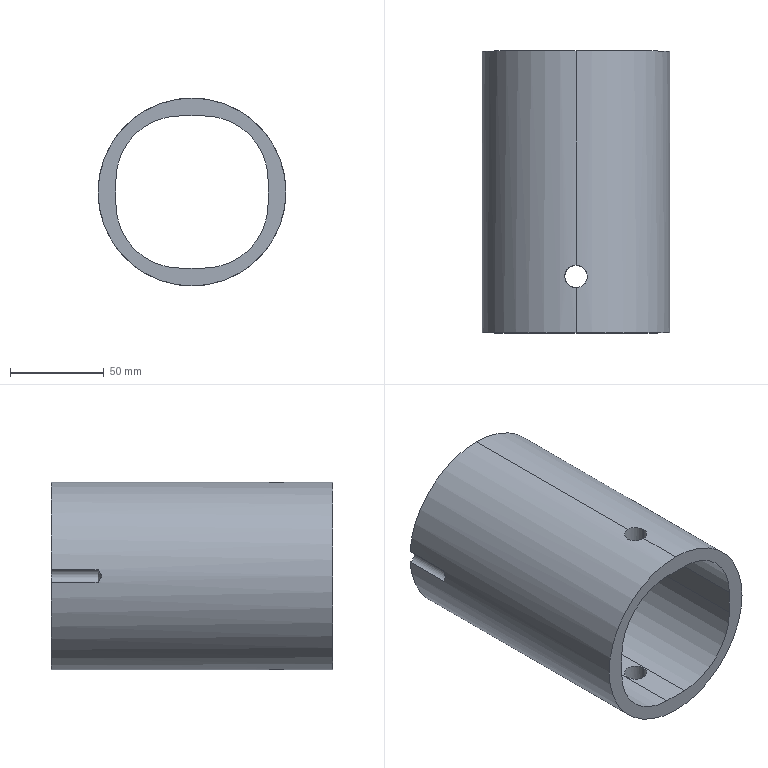Part | SolidWorks | features MirrorStock 1 | 1 solid | 20 faces | box 100 x 150 x 100 mm | volume 339747 mm3 | cylinder 12 | plane 6 | cone 2 | commonest cylinder face diameters 12 x4 68 x4 6.8 x2 100 x2
STEP:
#1=CARTESIAN_POINT('',(-6.,-45.,-40.5));
#2=VERTEX_POINT('',#1);
#3=CARTESIAN_POINT('',(6.,-45.,-40.5));
#4=VERTEX_POINT('',#3);
#5=CARTESIAN_POINT('',(0.,-45.,-40.5));
#6=DIRECTION('',(0.,0.,-1.));
#7=DIRECTION('',(-1.,0.,0.));
#8=AXIS2_PLACEMENT_3D('',#5,#6,#7);
#9=CIRCLE('',#8,6.);
#10=EDGE_CURVE('',#2,#4,#9,.T.);
#11=ORIENTED_EDGE('',*,*,#10,.F.);
#12=CARTESIAN_POINT('',(-6.,-45.,-49.639));
#13=VERTEX_POINT('',#12);
#14=CARTESIAN_POINT('',(-6.,-45.,75.));
#15=DIRECTION('',(0.,0.,-1.));
#16=VECTOR('',#15,1000.);
#17=LINE('',#14,#16);
#18=EDGE_CURVE('',#2,#13,#17,.T.);
#19=ORIENTED_EDGE('',*,*,#18,.T.);
#20=CARTESIAN_POINT('',(0.,-39.,-50.));
#21=VERTEX_POINT('',#20);
#22=CARTESIAN_POINT('',(-6.,-45.,-49.639));
#23=CARTESIAN_POINT('',(-6.,-44.608,-49.639));
#24=CARTESIAN_POINT('',(-5.962,-44.218,-49.643));
#25=CARTESIAN_POINT('',(-5.847,-43.637,-49.657));
#26=CARTESIAN_POINT('',(-5.798,-43.444,-49.663));
#27=CARTESIAN_POINT('',(-5.684,-43.068,-49.676));
#28=CARTESIAN_POINT('',(-5.552,-42.7,-49.691));
#29=CARTESIAN_POINT('',(-5.385,-42.346,-49.709));
#30=CARTESIAN_POINT('',(-5.2,-42.,-49.729));
#31=CARTESIAN_POINT('',(-5.098,-41.829,-49.74));
#32=CARTESIAN_POINT('',(-4.769,-41.337,-49.773));
#33=CARTESIAN_POINT('',(-4.521,-41.035,-49.796));
#34=CARTESIAN_POINT('',(-3.967,-40.482,-49.843));
#35=CARTESIAN_POINT('',(-3.659,-40.229,-49.867));
#36=CARTESIAN_POINT('',(-3.007,-39.793,-49.911));
#37=CARTESIAN_POINT('',(-2.663,-39.609,-49.93));
#38=CARTESIAN_POINT('',(-2.117,-39.383,-49.955));
#39=CARTESIAN_POINT('',(-1.93,-39.315,-49.963));
#40=CARTESIAN_POINT('',(-1.553,-39.201,-49.976));
#41=CARTESIAN_POINT('',(-1.363,-39.154,-49.982));
#42=CARTESIAN_POINT('',(-0.7871,-39.039,-49.995));
#43=CARTESIAN_POINT('',(-0.3969,-39.,-50.));
#44=CARTESIAN_POINT('',(0.,-39.,-50.));
#45=B_SPLINE_CURVE_WITH_KNOTS('',3,(#22,#23,#24,#25,#26,#27,#28,#29,#30,#31,#32,#33,#34,#35,#36,#37,#38,#39,#40,#41,#42,#43,#44),.UNSPECIFIED.,.F.,.F.,(4,2,2,1,2,2,2,2,2,2,2,4),(0.01878,0.01995,0.02054,0.02112,0.02171,0.0223,0.02347,0.02464,0.02582,0.0264,0.02699,0.02817),.UNSPECIFIED.);
#46=EDGE_CURVE('',#13,#21,#45,.T.);
#47=ORIENTED_EDGE('',*,*,#46,.T.);
#48=CARTESIAN_POINT('',(6.,-45.,-49.639));
#49=VERTEX_POINT('',#48);
#50=CARTESIAN_POINT('',(0.,-39.,-50.));
#51=CARTESIAN_POINT('',(0.3965,-39.,-50.));
#52=CARTESIAN_POINT('',(0.7864,-39.039,-49.995));
#53=CARTESIAN_POINT('',(1.362,-39.153,-49.982));
#54=CARTESIAN_POINT('',(1.552,-39.201,-49.976));
#55=CARTESIAN_POINT('',(1.929,-39.315,-49.963));
#56=CARTESIAN_POINT('',(2.116,-39.382,-49.956));
#57=CARTESIAN_POINT('',(2.66,-39.608,-49.93));
#58=CARTESIAN_POINT('',(3.005,-39.792,-49.911));
#59=CARTESIAN_POINT('',(3.657,-40.227,-49.867));
#60=CARTESIAN_POINT('',(3.965,-40.48,-49.843));
#61=CARTESIAN_POINT('',(4.518,-41.032,-49.796));
#62=CARTESIAN_POINT('',(4.766,-41.334,-49.773));
#63=CARTESIAN_POINT('',(5.095,-41.825,-49.74));
#64=CARTESIAN_POINT('',(5.197,-41.995,-49.729));
#65=CARTESIAN_POINT('',(5.382,-42.341,-49.71));
#66=CARTESIAN_POINT('',(5.466,-42.517,-49.7));
#67=CARTESIAN_POINT('',(5.691,-43.058,-49.675));
#68=CARTESIAN_POINT('',(5.806,-43.436,-49.662));
#69=CARTESIAN_POINT('',(5.961,-44.211,-49.643));
#70=CARTESIAN_POINT('',(6.,-44.603,-49.639));
#71=CARTESIAN_POINT('',(6.,-45.,-49.639));
#72=B_SPLINE_CURVE_WITH_KNOTS('',3,(#50,#51,#52,#53,#54,#55,#56,#57,#58,#59,#60,#61,#62,#63,#64,#65,#66,#67,#68,#69,#70,#71),.UNSPECIFIED.,.F.,.F.,(4,2,2,2,2,2,2,2,2,2,4),(0.02817,0.02934,0.02992,0.03051,0.03168,0.03286,0.03403,0.03462,0.0352,0.03637,0.03755),.UNSPECIFIED.);
#73=EDGE_CURVE('',#21,#49,#72,.T.);
#74=ORIENTED_EDGE('',*,*,#73,.T.);
#75=CARTESIAN_POINT('',(6.,-45.,75.));
#76=DIRECTION('',(0.,0.,-1.));
#77=VECTOR('',#76,1000.);
#78=LINE('',#75,#77);
#79=EDGE_CURVE('',#4,#49,#78,.T.);
#80=ORIENTED_EDGE('',*,*,#79,.F.);
#81=EDGE_LOOP('',(#11,#19,#47,#74,#80));
#82=FACE_OUTER_BOUND('',#81,.T.);
#83=CARTESIAN_POINT('',(0.,-45.,75.));
#84=DIRECTION('',(0.,0.,-1.));
#85=DIRECTION('',(1.,0.,0.));
#86=AXIS2_PLACEMENT_3D('',#83,#84,#85);
#87=CYLINDRICAL_SURFACE('',#86,6.);
#88=ADVANCED_FACE('',(#82),#87,.F.);
#89=CARTESIAN_POINT('',(0.,-39.,50.));
#90=VERTEX_POINT('',#89);
#91=CARTESIAN_POINT('',(-6.,-45.,49.639));
#92=VERTEX_POINT('',#91);
#93=CARTESIAN_POINT('',(0.,-39.,50.));
#94=CARTESIAN_POINT('',(-0.3969,-39.,50.));
#95=CARTESIAN_POINT('',(-0.7871,-39.039,49.995));
#96=CARTESIAN_POINT('',(-1.363,-39.154,49.982));
#97=CARTESIAN_POINT('',(-1.553,-39.201,49.976));
#98=CARTESIAN_POINT('',(-1.93,-39.316,49.963));
#99=CARTESIAN_POINT('',(-2.118,-39.383,49.955));
#100=CARTESIAN_POINT('',(-2.663,-39.609,49.93));
#101=CARTESIAN_POINT('',(-3.007,-39.793,49.911));
#102=CARTESIAN_POINT('',(-3.659,-40.229,49.867));
#103=CARTESIAN_POINT('',(-3.968,-40.482,49.843));
#104=CARTESIAN_POINT('',(-4.521,-41.036,49.796));
#105=CARTESIAN_POINT('',(-4.769,-41.338,49.773));
#106=CARTESIAN_POINT('',(-5.098,-41.83,49.74));
#107=CARTESIAN_POINT('',(-5.2,-42.,49.729));
#108=CARTESIAN_POINT('',(-5.385,-42.346,49.709));
#109=CARTESIAN_POINT('',(-5.552,-42.7,49.691));
#110=CARTESIAN_POINT('',(-5.684,-43.069,49.676));
#111=CARTESIAN_POINT('',(-5.798,-43.444,49.663));
#112=CARTESIAN_POINT('',(-5.847,-43.637,49.657));
#113=CARTESIAN_POINT('',(-5.962,-44.218,49.643));
#114=CARTESIAN_POINT('',(-6.,-44.608,49.639));
#115=CARTESIAN_POINT('',(-6.,-45.,49.639));
#116=B_SPLINE_CURVE_WITH_KNOTS('',3,(#93,#94,#95,#96,#97,#98,#99,#100,#101,#102,#103,#104,#105,#106,#107,#108,#109,#110,#111,#112,#113,#114,#115),.UNSPECIFIED.,.F.,.F.,(4,2,2,2,2,2,2,2,1,2,2,4),(0.,0.001174,0.001761,0.002348,0.003521,0.004695,0.005869,0.006456,0.007043,0.007629,0.008216,0.00939),.UNSPECIFIED.);
#117=EDGE_CURVE('',#90,#92,#116,.T.);
#118=ORIENTED_EDGE('',*,*,#117,.T.);
#119=CARTESIAN_POINT('',(-6.,-45.,40.5));
#120=VERTEX_POINT('',#119);
#121=CARTESIAN_POINT('',(-6.,-45.,75.));
#122=DIRECTION('',(0.,0.,-1.));
#123=VECTOR('',#122,1000.);
#124=LINE('',#121,#123);
#125=EDGE_CURVE('',#92,#120,#124,.T.);
#126=ORIENTED_EDGE('',*,*,#125,.T.);
#127=CARTESIAN_POINT('',(6.,-45.,40.5));
#128=VERTEX_POINT('',#127);
#129=CARTESIAN_POINT('',(0.,-45.,40.5));
#130=DIRECTION('',(0.,0.,1.));
#131=DIRECTION('',(1.,0.,0.));
#132=AXIS2_PLACEMENT_3D('',#129,#130,#131);
#133=CIRCLE('',#132,6.);
#134=EDGE_CURVE('',#128,#120,#133,.T.);
#135=ORIENTED_EDGE('',*,*,#134,.F.);
#136=CARTESIAN_POINT('',(6.,-45.,49.639));
#137=VERTEX_POINT('',#136);
#138=CARTESIAN_POINT('',(6.,-45.,75.));
#139=DIRECTION('',(0.,0.,-1.));
#140=VECTOR('',#139,1000.);
#141=LINE('',#138,#140);
#142=EDGE_CURVE('',#137,#128,#141,.T.);
#143=ORIENTED_EDGE('',*,*,#142,.F.);
#144=CARTESIAN_POINT('',(6.,-45.,49.639));
#145=CARTESIAN_POINT('',(6.,-44.603,49.639));
#146=CARTESIAN_POINT('',(5.961,-44.214,49.643));
#147=CARTESIAN_POINT('',(5.847,-43.638,49.657));
#148=CARTESIAN_POINT('',(5.799,-43.448,49.663));
#149=CARTESIAN_POINT('',(5.685,-43.071,49.676));
#150=CARTESIAN_POINT('',(5.618,-42.884,49.683));
#151=CARTESIAN_POINT('',(5.392,-42.34,49.709));
#152=CARTESIAN_POINT('',(5.208,-41.995,49.728));
#153=CARTESIAN_POINT('',(4.773,-41.343,49.772));
#154=CARTESIAN_POINT('',(4.52,-41.035,49.796));
#155=CARTESIAN_POINT('',(3.968,-40.482,49.843));
#156=CARTESIAN_POINT('',(3.666,-40.234,49.866));
#157=CARTESIAN_POINT('',(3.175,-39.905,49.899));
#158=CARTESIAN_POINT('',(3.005,-39.803,49.91));
#159=CARTESIAN_POINT('',(2.659,-39.618,49.93));
#160=CARTESIAN_POINT('',(2.483,-39.534,49.939));
#161=CARTESIAN_POINT('',(1.942,-39.309,49.964));
#162=CARTESIAN_POINT('',(1.564,-39.194,49.977));
#163=CARTESIAN_POINT('',(0.7886,-39.039,49.995));
#164=CARTESIAN_POINT('',(0.3965,-39.,50.));
#165=CARTESIAN_POINT('',(0.,-39.,50.));
#166=B_SPLINE_CURVE_WITH_KNOTS('',3,(#144,#145,#146,#147,#148,#149,#150,#151,#152,#153,#154,#155,#156,#157,#158,#159,#160,#161,#162,#163,#164,#165),.UNSPECIFIED.,.F.,.F.,(4,2,2,2,2,2,2,2,2,2,4),(0.02817,0.02934,0.02992,0.03051,0.03168,0.03286,0.03403,0.03462,0.0352,0.03637,0.03755),.UNSPECIFIED.);
#167=EDGE_CURVE('',#137,#90,#166,.T.);
#168=ORIENTED_EDGE('',*,*,#167,.T.);
#169=EDGE_LOOP('',(#118,#126,#135,#143,#168));
#170=FACE_OUTER_BOUND('',#169,.T.);
#171=CARTESIAN_POINT('',(0.,-45.,75.));
#172=DIRECTION('',(0.,0.,-1.));
#173=DIRECTION('',(1.,0.,0.));
#174=AXIS2_PLACEMENT_3D('',#171,#172,#173);
#175=CYLINDRICAL_SURFACE('',#174,6.);
#176=ADVANCED_FACE('',(#170),#175,.F.);
#177=CARTESIAN_POINT('',(-49.884,75.,-3.398));
#178=VERTEX_POINT('',#177);
#179=CARTESIAN_POINT('',(0.,75.,-50.));
#180=VERTEX_POINT('',#179);
#181=CARTESIAN_POINT('',(0.,75.,0.));
#182=DIRECTION('',(0.,-1.,0.));
#183=DIRECTION('',(0.,0.,-1.));
#184=AXIS2_PLACEMENT_3D('',#181,#182,#183);
#185=CIRCLE('',#184,50.);
#186=EDGE_CURVE('',#178,#180,#185,.T.);
#187=ORIENTED_EDGE('',*,*,#186,.T.);
#188=CARTESIAN_POINT('',(0.,75.,-50.));
#189=DIRECTION('',(0.,-1.,0.));
#190=VECTOR('',#189,1000.);
#191=LINE('',#188,#190);
#192=EDGE_CURVE('',#180,#21,#191,.T.);
#193=ORIENTED_EDGE('',*,*,#192,.T.);
#194=ORIENTED_EDGE('',*,*,#46,.F.);
#195=CARTESIAN_POINT('',(0.,-51.,-50.));
#196=VERTEX_POINT('',#195);
#197=CARTESIAN_POINT('',(0.,-51.,-50.));
#198=CARTESIAN_POINT('',(-0.3917,-51.,-50.));
#199=CARTESIAN_POINT('',(-0.7895,-50.961,-49.995));
#200=CARTESIAN_POINT('',(-1.559,-50.807,-49.977));
#201=CARTESIAN_POINT('',(-1.933,-50.694,-49.964));
#202=CARTESIAN_POINT('',(-2.478,-50.468,-49.939));
#203=CARTESIAN_POINT('',(-2.658,-50.383,-49.93));
#204=CARTESIAN_POINT('',(-3.005,-50.197,-49.91));
#205=CARTESIAN_POINT('',(-3.173,-50.096,-49.899));
#206=CARTESIAN_POINT('',(-3.66,-49.77,-49.867));
#207=CARTESIAN_POINT('',(-3.963,-49.522,-49.843));
#208=CARTESIAN_POINT('',(-4.523,-48.962,-49.796));
#209=CARTESIAN_POINT('',(-4.771,-48.66,-49.772));
#210=CARTESIAN_POINT('',(-5.096,-48.173,-49.74));
#211=CARTESIAN_POINT('',(-5.197,-48.005,-49.729));
#212=CARTESIAN_POINT('',(-5.383,-47.658,-49.709));
#213=CARTESIAN_POINT('',(-5.468,-47.478,-49.7));
#214=CARTESIAN_POINT('',(-5.694,-46.933,-49.675));
#215=CARTESIAN_POINT('',(-5.807,-46.559,-49.662));
#216=CARTESIAN_POINT('',(-5.961,-45.79,-49.643));
#217=CARTESIAN_POINT('',(-6.,-45.392,-49.639));
#218=CARTESIAN_POINT('',(-6.,-45.,-49.639));
#219=B_SPLINE_CURVE_WITH_KNOTS('',3,(#197,#198,#199,#200,#201,#202,#203,#204,#205,#206,#207,#208,#209,#210,#211,#212,#213,#214,#215,#216,#217,#218),.UNSPECIFIED.,.F.,.F.,(4,2,2,2,2,2,2,2,2,2,4),(0.00939,0.01056,0.01174,0.01232,0.01291,0.01408,0.01526,0.01584,0.01643,0.0176,0.01878),.UNSPECIFIED.);
#220=EDGE_CURVE('',#196,#13,#219,.T.);
#221=ORIENTED_EDGE('',*,*,#220,.F.);
#222=CARTESIAN_POINT('',(0.,-75.,-50.));
#223=VERTEX_POINT('',#222);
#224=CARTESIAN_POINT('',(0.,75.,-50.));
#225=DIRECTION('',(0.,-1.,0.));
#226=VECTOR('',#225,1000.);
#227=LINE('',#224,#226);
#228=EDGE_CURVE('',#196,#223,#227,.T.);
#229=ORIENTED_EDGE('',*,*,#228,.T.);
#230=CARTESIAN_POINT('',(0.,-75.,50.));
#231=VERTEX_POINT('',#230);
#232=CARTESIAN_POINT('',(0.,-75.,0.));
#233=DIRECTION('',(0.,-1.,0.));
#234=DIRECTION('',(0.,0.,-1.));
#235=AXIS2_PLACEMENT_3D('',#232,#233,#234);
#236=CIRCLE('',#235,50.);
#237=EDGE_CURVE('',#231,#223,#236,.T.);
#238=ORIENTED_EDGE('',*,*,#237,.F.);
#239=CARTESIAN_POINT('',(0.,-51.,50.));
#240=VERTEX_POINT('',#239);
#241=CARTESIAN_POINT('',(0.,75.,50.));
#242=DIRECTION('',(0.,-1.,0.));
#243=VECTOR('',#242,1000.);
#244=LINE('',#241,#243);
#245=EDGE_CURVE('',#240,#231,#244,.T.);
#246=ORIENTED_EDGE('',*,*,#245,.F.);
#247=CARTESIAN_POINT('',(-6.,-45.,49.639));
#248=CARTESIAN_POINT('',(-6.,-45.392,49.639));
#249=CARTESIAN_POINT('',(-5.961,-45.789,49.643));
#250=CARTESIAN_POINT('',(-5.807,-46.559,49.662));
#251=CARTESIAN_POINT('',(-5.694,-46.933,49.675));
#252=CARTESIAN_POINT('',(-5.468,-47.478,49.7));
#253=CARTESIAN_POINT('',(-5.383,-47.658,49.71));
#254=CARTESIAN_POINT('',(-5.197,-48.005,49.729));
#255=CARTESIAN_POINT('',(-5.096,-48.173,49.74));
#256=CARTESIAN_POINT('',(-4.77,-48.66,49.772));
#257=CARTESIAN_POINT('',(-4.522,-48.963,49.796));
#258=CARTESIAN_POINT('',(-3.962,-49.523,49.844));
#259=CARTESIAN_POINT('',(-3.66,-49.771,49.867));
#260=CARTESIAN_POINT('',(-3.173,-50.096,49.9));
#261=CARTESIAN_POINT('',(-3.005,-50.197,49.91));
#262=CARTESIAN_POINT('',(-2.658,-50.383,49.93));
#263=CARTESIAN_POINT('',(-2.478,-50.468,49.939));
#264=CARTESIAN_POINT('',(-1.933,-50.694,49.964));
#265=CARTESIAN_POINT('',(-1.559,-50.807,49.977));
#266=CARTESIAN_POINT('',(-0.7895,-50.961,49.995));
#267=CARTESIAN_POINT('',(-0.3917,-51.,50.));
#268=CARTESIAN_POINT('',(0.,-51.,50.));
#269=B_SPLINE_CURVE_WITH_KNOTS('',3,(#247,#248,#249,#250,#251,#252,#253,#254,#255,#256,#257,#258,#259,#260,#261,#262,#263,#264,#265,#266,#267,#268),.UNSPECIFIED.,.F.,.F.,(4,2,2,2,2,2,2,2,2,2,4),(0.00939,0.01056,0.01174,0.01232,0.01291,0.01408,0.01526,0.01584,0.01643,0.0176,0.01878),.UNSPECIFIED.);
#270=EDGE_CURVE('',#92,#240,#269,.T.);
#271=ORIENTED_EDGE('',*,*,#270,.F.);
#272=ORIENTED_EDGE('',*,*,#117,.F.);
#273=CARTESIAN_POINT('',(0.,75.,50.));
#274=VERTEX_POINT('',#273);
#275=CARTESIAN_POINT('',(0.,75.,50.));
#276=DIRECTION('',(0.,-1.,0.));
#277=VECTOR('',#276,1000.);
#278=LINE('',#275,#277);
#279=EDGE_CURVE('',#274,#90,#278,.T.);
#280=ORIENTED_EDGE('',*,*,#279,.F.);
#281=CARTESIAN_POINT('',(-49.884,75.,3.398));
#282=VERTEX_POINT('',#281);
#283=CARTESIAN_POINT('',(0.,75.,0.));
#284=DIRECTION('',(0.,-1.,0.));
#285=DIRECTION('',(0.,0.,-1.));
#286=AXIS2_PLACEMENT_3D('',#283,#284,#285);
#287=CIRCLE('',#286,50.);
#288=EDGE_CURVE('',#274,#282,#287,.T.);
#289=ORIENTED_EDGE('',*,*,#288,.T.);
#290=CARTESIAN_POINT('',(-49.884,50.,3.398));
#291=VERTEX_POINT('',#290);
#292=CARTESIAN_POINT('',(-49.884,62.5,3.398));
#293=DIRECTION('',(0.,1.,0.));
#294=VECTOR('',#293,1000.);
#295=LINE('',#292,#294);
#296=EDGE_CURVE('',#291,#282,#295,.T.);
#297=ORIENTED_EDGE('',*,*,#296,.F.);
#298=CARTESIAN_POINT('',(-50.,47.957,0.));
#299=VERTEX_POINT('',#298);
#300=CARTESIAN_POINT('',(-50.,47.957,0.));
#301=CARTESIAN_POINT('',(-50.,48.638,1.134));
#302=CARTESIAN_POINT('',(-49.961,49.319,2.267));
#303=CARTESIAN_POINT('',(-49.884,50.,3.398));
#304=B_SPLINE_CURVE_WITH_KNOTS('',3,(#300,#301,#302,#303),.UNSPECIFIED.,.F.,.F.,(4,4),(-0.000000022,0.003968),.UNSPECIFIED.);
#305=EDGE_CURVE('',#299,#291,#304,.T.);
#306=ORIENTED_EDGE('',*,*,#305,.F.);
#307=CARTESIAN_POINT('',(-49.884,50.,-3.398));
#308=VERTEX_POINT('',#307);
#309=CARTESIAN_POINT('',(-49.884,50.,-3.398));
#310=CARTESIAN_POINT('',(-49.961,49.319,-2.267));
#311=CARTESIAN_POINT('',(-50.,48.638,-1.133));
#312=CARTESIAN_POINT('',(-50.,47.957,0.));
#313=B_SPLINE_CURVE_WITH_KNOTS('',3,(#309,#310,#311,#312),.UNSPECIFIED.,.F.,.F.,(4,4),(0.0004031,0.00437),.UNSPECIFIED.);
#314=EDGE_CURVE('',#308,#299,#313,.T.);
#315=ORIENTED_EDGE('',*,*,#314,.F.);
#316=CARTESIAN_POINT('',(-49.884,62.5,-3.398));
#317=DIRECTION('',(0.,-1.,0.));
#318=VECTOR('',#317,1000.);
#319=LINE('',#316,#318);
#320=EDGE_CURVE('',#178,#308,#319,.T.);
#321=ORIENTED_EDGE('',*,*,#320,.F.);
#322=EDGE_LOOP('',(#187,#193,#194,#221,#229,#238,#246,#271,#272,#280,#289,#297,#306,#315,#321));
#323=FACE_OUTER_BOUND('',#322,.T.);
#324=CARTESIAN_POINT('',(0.,75.,0.));
#325=DIRECTION('',(0.,-1.,0.));
#326=DIRECTION('',(0.,0.,1.));
#327=AXIS2_PLACEMENT_3D('',#324,#325,#326);
#328=CYLINDRICAL_SURFACE('',#327,50.);
#329=ADVANCED_FACE('',(#323),#328,.T.);
#330=CARTESIAN_POINT('',(-50.,75.,0.));
#331=DIRECTION('',(0.,-1.,0.));
#332=DIRECTION('',(0.,0.,-1.));
#333=AXIS2_PLACEMENT_3D('',#330,#331,#332);
#334=CIRCLE('',#333,3.4);
#335=EDGE_CURVE('',#178,#282,#334,.T.);
#336=ORIENTED_EDGE('',*,*,#335,.T.);
#337=ORIENTED_EDGE('',*,*,#288,.F.);
#338=CARTESIAN_POINT('',(49.884,75.,3.398));
#339=VERTEX_POINT('',#338);
#340=CARTESIAN_POINT('',(0.,75.,0.));
#341=DIRECTION('',(0.,-1.,0.));
#342=DIRECTION('',(0.,0.,-1.));
#343=AXIS2_PLACEMENT_3D('',#340,#341,#342);
#344=CIRCLE('',#343,50.);
#345=EDGE_CURVE('',#339,#274,#344,.T.);
#346=ORIENTED_EDGE('',*,*,#345,.F.);
#347=CARTESIAN_POINT('',(49.884,75.,-3.398));
#348=VERTEX_POINT('',#347);
#349=CARTESIAN_POINT('',(50.,75.,0.));
#350=DIRECTION('',(0.,-1.,0.));
#351=DIRECTION('',(0.,0.,-1.));
#352=AXIS2_PLACEMENT_3D('',#349,#350,#351);
#353=CIRCLE('',#352,3.4);
#354=EDGE_CURVE('',#339,#348,#353,.T.);
#355=ORIENTED_EDGE('',*,*,#354,.T.);
#356=CARTESIAN_POINT('',(0.,75.,0.));
#357=DIRECTION('',(0.,-1.,0.));
#358=DIRECTION('',(0.,0.,-1.));
#359=AXIS2_PLACEMENT_3D('',#356,#357,#358);
#360=CIRCLE('',#359,50.);
#361=EDGE_CURVE('',#180,#348,#360,.T.);
#362=ORIENTED_EDGE('',*,*,#361,.F.);
#363=ORIENTED_EDGE('',*,*,#186,.F.);
#364=EDGE_LOOP('',(#336,#337,#346,#355,#362,#363));
#365=FACE_OUTER_BOUND('',#364,.T.);
#366=CARTESIAN_POINT('',(-6.5,75.,-40.5));
#367=VERTEX_POINT('',#366);
#368=CARTESIAN_POINT('',(6.5,75.,-40.5));
#369=VERTEX_POINT('',#368);
#370=CARTESIAN_POINT('',(-6.5,75.,-40.5));
#371=DIRECTION('',(1.,0.,0.));
#372=VECTOR('',#371,1000.);
#373=LINE('',#370,#372);
#374=EDGE_CURVE('',#367,#369,#373,.T.);
#375=ORIENTED_EDGE('',*,*,#374,.T.);
#376=CARTESIAN_POINT('',(40.5,75.,-6.5));
#377=VERTEX_POINT('',#376);
#378=CARTESIAN_POINT('',(6.5,75.,-6.5));
#379=DIRECTION('',(0.,-1.,0.));
#380=DIRECTION('',(0.,0.,-1.));
#381=AXIS2_PLACEMENT_3D('',#378,#379,#380);
#382=CIRCLE('',#381,34.);
#383=EDGE_CURVE('',#369,#377,#382,.T.);
#384=ORIENTED_EDGE('',*,*,#383,.T.);
#385=CARTESIAN_POINT('',(40.5,75.,6.5));
#386=VERTEX_POINT('',#385);
#387=CARTESIAN_POINT('',(40.5,75.,-6.5));
#388=DIRECTION('',(0.,0.,1.));
#389=VECTOR('',#388,1000.);
#390=LINE('',#387,#389);
#391=EDGE_CURVE('',#377,#386,#390,.T.);
#392=ORIENTED_EDGE('',*,*,#391,.T.);
#393=CARTESIAN_POINT('',(6.5,75.,40.5));
#394=VERTEX_POINT('',#393);
#395=CARTESIAN_POINT('',(6.5,75.,6.5));
#396=DIRECTION('',(0.,-1.,0.));
#397=DIRECTION('',(0.,0.,1.));
#398=AXIS2_PLACEMENT_3D('',#395,#396,#397);
#399=CIRCLE('',#398,34.);
#400=EDGE_CURVE('',#386,#394,#399,.T.);
#401=ORIENTED_EDGE('',*,*,#400,.T.);
#402=CARTESIAN_POINT('',(-6.5,75.,40.5));
#403=VERTEX_POINT('',#402);
#404=CARTESIAN_POINT('',(-6.5,75.,40.5));
#405=DIRECTION('',(-1.,0.,0.));
#406=VECTOR('',#405,1000.);
#407=LINE('',#404,#406);
#408=EDGE_CURVE('',#394,#403,#407,.T.);
#409=ORIENTED_EDGE('',*,*,#408,.T.);
#410=CARTESIAN_POINT('',(-40.5,75.,6.5));
#411=VERTEX_POINT('',#410);
#412=CARTESIAN_POINT('',(-6.5,75.,6.5));
#413=DIRECTION('',(0.,-1.,0.));
#414=DIRECTION('',(0.,0.,1.));
#415=AXIS2_PLACEMENT_3D('',#412,#413,#414);
#416=CIRCLE('',#415,34.);
#417=EDGE_CURVE('',#403,#411,#416,.T.);
#418=ORIENTED_EDGE('',*,*,#417,.T.);
#419=CARTESIAN_POINT('',(-40.5,75.,-6.5));
#420=VERTEX_POINT('',#419);
#421=CARTESIAN_POINT('',(-40.5,75.,-6.5));
#422=DIRECTION('',(0.,0.,-1.));
#423=VECTOR('',#422,1000.);
#424=LINE('',#421,#423);
#425=EDGE_CURVE('',#411,#420,#424,.T.);
#426=ORIENTED_EDGE('',*,*,#425,.T.);
#427=CARTESIAN_POINT('',(-6.5,75.,-6.5));
#428=DIRECTION('',(0.,-1.,0.));
#429=DIRECTION('',(0.,0.,1.));
#430=AXIS2_PLACEMENT_3D('',#427,#428,#429);
#431=CIRCLE('',#430,34.);
#432=EDGE_CURVE('',#420,#367,#431,.T.);
#433=ORIENTED_EDGE('',*,*,#432,.T.);
#434=EDGE_LOOP('',(#375,#384,#392,#401,#409,#418,#426,#433));
#435=FACE_BOUND('',#434,.T.);
#436=CARTESIAN_POINT('',(0.,75.,0.));
#437=DIRECTION('',(0.,1.,0.));
#438=DIRECTION('',(0.,0.,-1.));
#439=AXIS2_PLACEMENT_3D('',#436,#437,#438);
#440=PLANE('',#439);
#441=ADVANCED_FACE('',(#365,#435),#440,.T.);
#442=ORIENTED_EDGE('',*,*,#237,.T.);
#443=CARTESIAN_POINT('',(0.,-75.,0.));
#444=DIRECTION('',(0.,-1.,0.));
#445=DIRECTION('',(0.,0.,-1.));
#446=AXIS2_PLACEMENT_3D('',#443,#444,#445);
#447=CIRCLE('',#446,50.);
#448=EDGE_CURVE('',#223,#231,#447,.T.);
#449=ORIENTED_EDGE('',*,*,#448,.T.);
#450=EDGE_LOOP('',(#442,#449));
#451=FACE_OUTER_BOUND('',#450,.T.);
#452=CARTESIAN_POINT('',(-40.5,-75.,-6.5));
#453=VERTEX_POINT('',#452);
#454=CARTESIAN_POINT('',(-6.5,-75.,-40.5));
#455=VERTEX_POINT('',#454);
#456=CARTESIAN_POINT('',(-6.5,-75.,-6.5));
#457=DIRECTION('',(0.,-1.,0.));
#458=DIRECTION('',(0.,0.,1.));
#459=AXIS2_PLACEMENT_3D('',#456,#457,#458);
#460=CIRCLE('',#459,34.);
#461=EDGE_CURVE('',#453,#455,#460,.T.);
#462=ORIENTED_EDGE('',*,*,#461,.F.);
#463=CARTESIAN_POINT('',(-40.5,-75.,6.5));
#464=VERTEX_POINT('',#463);
#465=CARTESIAN_POINT('',(-40.5,-75.,-6.5));
#466=DIRECTION('',(0.,0.,-1.));
#467=VECTOR('',#466,1000.);
#468=LINE('',#465,#467);
#469=EDGE_CURVE('',#464,#453,#468,.T.);
#470=ORIENTED_EDGE('',*,*,#469,.F.);
#471=CARTESIAN_POINT('',(-6.5,-75.,40.5));
#472=VERTEX_POINT('',#471);
#473=CARTESIAN_POINT('',(-6.5,-75.,6.5));
#474=DIRECTION('',(0.,-1.,0.));
#475=DIRECTION('',(0.,0.,1.));
#476=AXIS2_PLACEMENT_3D('',#473,#474,#475);
#477=CIRCLE('',#476,34.);
#478=EDGE_CURVE('',#472,#464,#477,.T.);
#479=ORIENTED_EDGE('',*,*,#478,.F.);
#480=CARTESIAN_POINT('',(6.5,-75.,40.5));
#481=VERTEX_POINT('',#480);
#482=CARTESIAN_POINT('',(-6.5,-75.,40.5));
#483=DIRECTION('',(-1.,0.,0.));
#484=VECTOR('',#483,1000.);
#485=LINE('',#482,#484);
#486=EDGE_CURVE('',#481,#472,#485,.T.);
#487=ORIENTED_EDGE('',*,*,#486,.F.);
#488=CARTESIAN_POINT('',(40.5,-75.,6.5));
#489=VERTEX_POINT('',#488);
#490=CARTESIAN_POINT('',(6.5,-75.,6.5));
#491=DIRECTION('',(0.,-1.,0.));
#492=DIRECTION('',(0.,0.,1.));
#493=AXIS2_PLACEMENT_3D('',#490,#491,#492);
#494=CIRCLE('',#493,34.);
#495=EDGE_CURVE('',#489,#481,#494,.T.);
#496=ORIENTED_EDGE('',*,*,#495,.F.);
#497=CARTESIAN_POINT('',(40.5,-75.,-6.5));
#498=VERTEX_POINT('',#497);
#499=CARTESIAN_POINT('',(40.5,-75.,-6.5));
#500=DIRECTION('',(0.,0.,1.));
#501=VECTOR('',#500,1000.);
#502=LINE('',#499,#501);
#503=EDGE_CURVE('',#498,#489,#502,.T.);
#504=ORIENTED_EDGE('',*,*,#503,.F.);
#505=CARTESIAN_POINT('',(6.5,-75.,-40.5));
#506=VERTEX_POINT('',#505);
#507=CARTESIAN_POINT('',(6.5,-75.,-6.5));
#508=DIRECTION('',(0.,-1.,0.));
#509=DIRECTION('',(0.,0.,-1.));
#510=AXIS2_PLACEMENT_3D('',#507,#508,#509);
#511=CIRCLE('',#510,34.);
#512=EDGE_CURVE('',#506,#498,#511,.T.);
#513=ORIENTED_EDGE('',*,*,#512,.F.);
#514=CARTESIAN_POINT('',(-6.5,-75.,-40.5));
#515=DIRECTION('',(1.,0.,0.));
#516=VECTOR('',#515,1000.);
#517=LINE('',#514,#516);
#518=EDGE_CURVE('',#455,#506,#517,.T.);
#519=ORIENTED_EDGE('',*,*,#518,.F.);
#520=EDGE_LOOP('',(#462,#470,#479,#487,#496,#504,#513,#519));
#521=FACE_BOUND('',#520,.T.);
#522=CARTESIAN_POINT('',(0.,-75.,0.));
#523=DIRECTION('',(0.,1.,0.));
#524=DIRECTION('',(0.,0.,-1.));
#525=AXIS2_PLACEMENT_3D('',#522,#523,#524);
#526=PLANE('',#525);
#527=ADVANCED_FACE('',(#451,#521),#526,.F.);
#528=ORIENTED_EDGE('',*,*,#192,.F.);
#529=ORIENTED_EDGE('',*,*,#361,.T.);
#530=CARTESIAN_POINT('',(49.884,50.,-3.398));
#531=VERTEX_POINT('',#530);
#532=CARTESIAN_POINT('',(49.884,62.5,-3.398));
#533=DIRECTION('',(0.,1.,0.));
#534=VECTOR('',#533,1000.);
#535=LINE('',#532,#534);
#536=EDGE_CURVE('',#531,#348,#535,.T.);
#537=ORIENTED_EDGE('',*,*,#536,.F.);
#538=CARTESIAN_POINT('',(50.,47.957,0.));
#539=VERTEX_POINT('',#538);
#540=CARTESIAN_POINT('',(50.,47.957,0.));
#541=CARTESIAN_POINT('',(50.,48.638,-1.134));
#542=CARTESIAN_POINT('',(49.961,49.319,-2.267));
#543=CARTESIAN_POINT('',(49.884,50.,-3.398));
#544=B_SPLINE_CURVE_WITH_KNOTS('',3,(#540,#541,#542,#543),.UNSPECIFIED.,.F.,.F.,(4,4),(-0.000000022,0.003968),.UNSPECIFIED.);
#545=EDGE_CURVE('',#539,#531,#544,.T.);
#546=ORIENTED_EDGE('',*,*,#545,.F.);
#547=CARTESIAN_POINT('',(49.884,50.,3.398));
#548=VERTEX_POINT('',#547);
#549=CARTESIAN_POINT('',(49.884,50.,3.398));
#550=CARTESIAN_POINT('',(49.961,49.319,2.267));
#551=CARTESIAN_POINT('',(50.,48.638,1.133));
#552=CARTESIAN_POINT('',(50.,47.957,0.));
#553=B_SPLINE_CURVE_WITH_KNOTS('',3,(#549,#550,#551,#552),.UNSPECIFIED.,.F.,.F.,(4,4),(0.0004031,0.00437),.UNSPECIFIED.);
#554=EDGE_CURVE('',#548,#539,#553,.T.);
#555=ORIENTED_EDGE('',*,*,#554,.F.);
#556=CARTESIAN_POINT('',(49.884,62.5,3.398));
#557=DIRECTION('',(0.,-1.,0.));
#558=VECTOR('',#557,1000.);
#559=LINE('',#556,#558);
#560=EDGE_CURVE('',#339,#548,#559,.T.);
#561=ORIENTED_EDGE('',*,*,#560,.F.);
#562=ORIENTED_EDGE('',*,*,#345,.T.);
#563=ORIENTED_EDGE('',*,*,#279,.T.);
#564=ORIENTED_EDGE('',*,*,#167,.F.);
#565=CARTESIAN_POINT('',(0.,-51.,50.));
#566=CARTESIAN_POINT('',(0.3919,-51.,50.));
#567=CARTESIAN_POINT('',(0.7816,-50.962,49.995));
#568=CARTESIAN_POINT('',(1.363,-50.847,49.982));
#569=CARTESIAN_POINT('',(1.556,-50.798,49.976));
#570=CARTESIAN_POINT('',(1.932,-50.684,49.963));
#571=CARTESIAN_POINT('',(2.3,-50.552,49.948));
#572=CARTESIAN_POINT('',(2.654,-50.385,49.93));
#573=CARTESIAN_POINT('',(3.,-50.2,49.91));
#574=CARTESIAN_POINT('',(3.171,-50.098,49.9));
#575=CARTESIAN_POINT('',(3.663,-49.769,49.867));
#576=CARTESIAN_POINT('',(3.965,-49.521,49.843));
#577=CARTESIAN_POINT('',(4.518,-48.967,49.796));
#578=CARTESIAN_POINT('',(4.771,-48.659,49.772));
#579=CARTESIAN_POINT('',(5.207,-48.007,49.729));
#580=CARTESIAN_POINT('',(5.391,-47.663,49.709));
#581=CARTESIAN_POINT('',(5.617,-47.117,49.684));
#582=CARTESIAN_POINT('',(5.685,-46.93,49.676));
#583=CARTESIAN_POINT('',(5.799,-46.553,49.663));
#584=CARTESIAN_POINT('',(5.846,-46.363,49.657));
#585=CARTESIAN_POINT('',(5.961,-45.787,49.643));
#586=CARTESIAN_POINT('',(6.,-45.397,49.639));
#587=CARTESIAN_POINT('',(6.,-45.,49.639));
#588=B_SPLINE_CURVE_WITH_KNOTS('',3,(#565,#566,#567,#568,#569,#570,#571,#572,#573,#574,#575,#576,#577,#578,#579,#580,#581,#582,#583,#584,#585,#586,#587),.UNSPECIFIED.,.F.,.F.,(4,2,2,1,2,2,2,2,2,2,2,4),(0.01878,0.01995,0.02054,0.02112,0.02171,0.0223,0.02347,0.02464,0.02582,0.0264,0.02699,0.02817),.UNSPECIFIED.);
#589=EDGE_CURVE('',#240,#137,#588,.T.);
#590=ORIENTED_EDGE('',*,*,#589,.F.);
#591=ORIENTED_EDGE('',*,*,#245,.T.);
#592=ORIENTED_EDGE('',*,*,#448,.F.);
#593=ORIENTED_EDGE('',*,*,#228,.F.);
#594=CARTESIAN_POINT('',(6.,-45.,-49.639));
#595=CARTESIAN_POINT('',(6.,-45.397,-49.639));
#596=CARTESIAN_POINT('',(5.961,-45.787,-49.643));
#597=CARTESIAN_POINT('',(5.846,-46.363,-49.657));
#598=CARTESIAN_POINT('',(5.799,-46.553,-49.663));
#599=CARTESIAN_POINT('',(5.684,-46.93,-49.676));
#600=CARTESIAN_POINT('',(5.617,-47.118,-49.684));
#601=CARTESIAN_POINT('',(5.391,-47.663,-49.709));
#602=CARTESIAN_POINT('',(5.207,-48.007,-49.729));
#603=CARTESIAN_POINT('',(4.771,-48.659,-49.772));
#604=CARTESIAN_POINT('',(4.518,-48.968,-49.796));
#605=CARTESIAN_POINT('',(3.964,-49.521,-49.843));
#606=CARTESIAN_POINT('',(3.662,-49.769,-49.867));
#607=CARTESIAN_POINT('',(3.17,-50.098,-49.9));
#608=CARTESIAN_POINT('',(3.,-50.2,-49.91));
#609=CARTESIAN_POINT('',(2.654,-50.385,-49.93));
#610=CARTESIAN_POINT('',(2.3,-50.552,-49.948));
#611=CARTESIAN_POINT('',(1.931,-50.684,-49.963));
#612=CARTESIAN_POINT('',(1.556,-50.798,-49.976));
#613=CARTESIAN_POINT('',(1.363,-50.847,-49.982));
#614=CARTESIAN_POINT('',(0.7815,-50.962,-49.995));
#615=CARTESIAN_POINT('',(0.3918,-51.,-50.));
#616=CARTESIAN_POINT('',(0.,-51.,-50.));
#617=B_SPLINE_CURVE_WITH_KNOTS('',3,(#594,#595,#596,#597,#598,#599,#600,#601,#602,#603,#604,#605,#606,#607,#608,#609,#610,#611,#612,#613,#614,#615,#616),.UNSPECIFIED.,.F.,.F.,(4,2,2,2,2,2,2,2,1,2,2,4),(0.,0.001174,0.001761,0.002348,0.003521,0.004695,0.005869,0.006456,0.007043,0.007629,0.008216,0.00939),.UNSPECIFIED.);
#618=EDGE_CURVE('',#49,#196,#617,.T.);
#619=ORIENTED_EDGE('',*,*,#618,.F.);
#620=ORIENTED_EDGE('',*,*,#73,.F.);
#621=EDGE_LOOP('',(#528,#529,#537,#546,#555,#561,#562,#563,#564,#590,#591,#592,#593,#619,#620));
#622=FACE_OUTER_BOUND('',#621,.T.);
#623=CARTESIAN_POINT('',(0.,75.,0.));
#624=DIRECTION('',(0.,-1.,0.));
#625=DIRECTION('',(0.,0.,1.));
#626=AXIS2_PLACEMENT_3D('',#623,#624,#625);
#627=CYLINDRICAL_SURFACE('',#626,50.);
#628=ADVANCED_FACE('',(#622),#627,.T.);
#629=ORIENTED_EDGE('',*,*,#461,.T.);
#630=CARTESIAN_POINT('',(-6.5,75.,-40.5));
#631=DIRECTION('',(0.,-1.,0.));
#632=VECTOR('',#631,1000.);
#633=LINE('',#630,#632);
#634=EDGE_CURVE('',#367,#455,#633,.T.);
#635=ORIENTED_EDGE('',*,*,#634,.F.);
#636=ORIENTED_EDGE('',*,*,#432,.F.);
#637=CARTESIAN_POINT('',(-40.5,75.,-6.5));
#638=DIRECTION('',(0.,-1.,0.));
#639=VECTOR('',#638,1000.);
#640=LINE('',#637,#639);
#641=EDGE_CURVE('',#420,#453,#640,.T.);
#642=ORIENTED_EDGE('',*,*,#641,.T.);
#643=EDGE_LOOP('',(#629,#635,#636,#642));
#644=FACE_OUTER_BOUND('',#643,.T.);
#645=CARTESIAN_POINT('',(-6.5,75.,-6.5));
#646=DIRECTION('',(0.,-1.,0.));
#647=DIRECTION('',(0.,0.,1.));
#648=AXIS2_PLACEMENT_3D('',#645,#646,#647);
#649=CYLINDRICAL_SURFACE('',#648,34.);
#650=ADVANCED_FACE('',(#644),#649,.F.);
#651=CARTESIAN_POINT('',(0.,-45.,-40.5));
#652=DIRECTION('',(0.,0.,-1.));
#653=DIRECTION('',(-1.,0.,0.));
#654=AXIS2_PLACEMENT_3D('',#651,#652,#653);
#655=CIRCLE('',#654,6.);
#656=EDGE_CURVE('',#4,#2,#655,.T.);
#657=ORIENTED_EDGE('',*,*,#656,.T.);
#658=ORIENTED_EDGE('',*,*,#10,.T.);
#659=EDGE_LOOP('',(#657,#658));
#660=FACE_BOUND('',#659,.T.);
#661=ORIENTED_EDGE('',*,*,#518,.T.);
#662=CARTESIAN_POINT('',(6.5,75.,-40.5));
#663=DIRECTION('',(0.,-1.,0.));
#664=VECTOR('',#663,1000.);
#665=LINE('',#662,#664);
#666=EDGE_CURVE('',#369,#506,#665,.T.);
#667=ORIENTED_EDGE('',*,*,#666,.F.);
#668=ORIENTED_EDGE('',*,*,#374,.F.);
#669=ORIENTED_EDGE('',*,*,#634,.T.);
#670=EDGE_LOOP('',(#661,#667,#668,#669));
#671=FACE_OUTER_BOUND('',#670,.T.);
#672=CARTESIAN_POINT('',(-6.5,75.,-40.5));
#673=DIRECTION('',(0.,0.,1.));
#674=DIRECTION('',(-1.,0.,0.));
#675=AXIS2_PLACEMENT_3D('',#672,#673,#674);
#676=PLANE('',#675);
#677=ADVANCED_FACE('',(#660,#671),#676,.T.);
#678=ORIENTED_EDGE('',*,*,#512,.T.);
#679=CARTESIAN_POINT('',(40.5,75.,-6.5));
#680=DIRECTION('',(0.,-1.,0.));
#681=VECTOR('',#680,1000.);
#682=LINE('',#679,#681);
#683=EDGE_CURVE('',#377,#498,#682,.T.);
#684=ORIENTED_EDGE('',*,*,#683,.F.);
#685=ORIENTED_EDGE('',*,*,#383,.F.);
#686=ORIENTED_EDGE('',*,*,#666,.T.);
#687=EDGE_LOOP('',(#678,#684,#685,#686));
#688=FACE_OUTER_BOUND('',#687,.T.);
#689=CARTESIAN_POINT('',(6.5,75.,-6.5));
#690=DIRECTION('',(0.,-1.,0.));
#691=DIRECTION('',(0.,0.,1.));
#692=AXIS2_PLACEMENT_3D('',#689,#690,#691);
#693=CYLINDRICAL_SURFACE('',#692,34.);
#694=ADVANCED_FACE('',(#688),#693,.F.);
#695=ORIENTED_EDGE('',*,*,#503,.T.);
#696=CARTESIAN_POINT('',(40.5,75.,6.5));
#697=DIRECTION('',(0.,-1.,0.));
#698=VECTOR('',#697,1000.);
#699=LINE('',#696,#698);
#700=EDGE_CURVE('',#386,#489,#699,.T.);
#701=ORIENTED_EDGE('',*,*,#700,.F.);
#702=ORIENTED_EDGE('',*,*,#391,.F.);
#703=ORIENTED_EDGE('',*,*,#683,.T.);
#704=EDGE_LOOP('',(#695,#701,#702,#703));
#705=FACE_OUTER_BOUND('',#704,.T.);
#706=CARTESIAN_POINT('',(40.5,75.,-6.5));
#707=DIRECTION('',(-1.,0.,0.));
#708=DIRECTION('',(0.,0.,-1.));
#709=AXIS2_PLACEMENT_3D('',#706,#707,#708);
#710=PLANE('',#709);
#711=ADVANCED_FACE('',(#705),#710,.T.);
#712=ORIENTED_EDGE('',*,*,#495,.T.);
#713=CARTESIAN_POINT('',(6.5,75.,40.5));
#714=DIRECTION('',(0.,-1.,0.));
#715=VECTOR('',#714,1000.);
#716=LINE('',#713,#715);
#717=EDGE_CURVE('',#394,#481,#716,.T.);
#718=ORIENTED_EDGE('',*,*,#717,.F.);
#719=ORIENTED_EDGE('',*,*,#400,.F.);
#720=ORIENTED_EDGE('',*,*,#700,.T.);
#721=EDGE_LOOP('',(#712,#718,#719,#720));
#722=FACE_OUTER_BOUND('',#721,.T.);
#723=CARTESIAN_POINT('',(6.5,75.,6.5));
#724=DIRECTION('',(0.,-1.,0.));
#725=DIRECTION('',(0.,0.,1.));
#726=AXIS2_PLACEMENT_3D('',#723,#724,#725);
#727=CYLINDRICAL_SURFACE('',#726,34.);
#728=ADVANCED_FACE('',(#722),#727,.F.);
#729=ORIENTED_EDGE('',*,*,#134,.T.);
#730=CARTESIAN_POINT('',(0.,-45.,40.5));
#731=DIRECTION('',(0.,0.,1.));
#732=DIRECTION('',(1.,0.,0.));
#733=AXIS2_PLACEMENT_3D('',#730,#731,#732);
#734=CIRCLE('',#733,6.);
#735=EDGE_CURVE('',#120,#128,#734,.T.);
#736=ORIENTED_EDGE('',*,*,#735,.T.);
#737=EDGE_LOOP('',(#729,#736));
#738=FACE_BOUND('',#737,.T.);
#739=ORIENTED_EDGE('',*,*,#486,.T.);
#740=CARTESIAN_POINT('',(-6.5,75.,40.5));
#741=DIRECTION('',(0.,-1.,0.));
#742=VECTOR('',#741,1000.);
#743=LINE('',#740,#742);
#744=EDGE_CURVE('',#403,#472,#743,.T.);
#745=ORIENTED_EDGE('',*,*,#744,.F.);
#746=ORIENTED_EDGE('',*,*,#408,.F.);
#747=ORIENTED_EDGE('',*,*,#717,.T.);
#748=EDGE_LOOP('',(#739,#745,#746,#747));
#749=FACE_OUTER_BOUND('',#748,.T.);
#750=CARTESIAN_POINT('',(-6.5,75.,40.5));
#751=DIRECTION('',(0.,0.,-1.));
#752=DIRECTION('',(1.,0.,0.));
#753=AXIS2_PLACEMENT_3D('',#750,#751,#752);
#754=PLANE('',#753);
#755=ADVANCED_FACE('',(#738,#749),#754,.T.);
#756=ORIENTED_EDGE('',*,*,#478,.T.);
#757=CARTESIAN_POINT('',(-40.5,75.,6.5));
#758=DIRECTION('',(0.,-1.,0.));
#759=VECTOR('',#758,1000.);
#760=LINE('',#757,#759);
#761=EDGE_CURVE('',#411,#464,#760,.T.);
#762=ORIENTED_EDGE('',*,*,#761,.F.);
#763=ORIENTED_EDGE('',*,*,#417,.F.);
#764=ORIENTED_EDGE('',*,*,#744,.T.);
#765=EDGE_LOOP('',(#756,#762,#763,#764));
#766=FACE_OUTER_BOUND('',#765,.T.);
#767=CARTESIAN_POINT('',(-6.5,75.,6.5));
#768=DIRECTION('',(0.,-1.,0.));
#769=DIRECTION('',(0.,0.,1.));
#770=AXIS2_PLACEMENT_3D('',#767,#768,#769);
#771=CYLINDRICAL_SURFACE('',#770,34.);
#772=ADVANCED_FACE('',(#766),#771,.F.);
#773=ORIENTED_EDGE('',*,*,#469,.T.);
#774=ORIENTED_EDGE('',*,*,#641,.F.);
#775=ORIENTED_EDGE('',*,*,#425,.F.);
#776=ORIENTED_EDGE('',*,*,#761,.T.);
#777=EDGE_LOOP('',(#773,#774,#775,#776));
#778=FACE_OUTER_BOUND('',#777,.T.);
#779=CARTESIAN_POINT('',(-40.5,75.,-6.5));
#780=DIRECTION('',(1.,0.,0.));
#781=DIRECTION('',(0.,0.,1.));
#782=AXIS2_PLACEMENT_3D('',#779,#780,#781);
#783=PLANE('',#782);
#784=ADVANCED_FACE('',(#778),#783,.T.);
#785=ORIENTED_EDGE('',*,*,#125,.F.);
#786=ORIENTED_EDGE('',*,*,#270,.T.);
#787=ORIENTED_EDGE('',*,*,#589,.T.);
#788=ORIENTED_EDGE('',*,*,#142,.T.);
#789=ORIENTED_EDGE('',*,*,#735,.F.);
#790=EDGE_LOOP('',(#785,#786,#787,#788,#789));
#791=FACE_OUTER_BOUND('',#790,.T.);
#792=CARTESIAN_POINT('',(0.,-45.,75.));
#793=DIRECTION('',(0.,0.,-1.));
#794=DIRECTION('',(1.,0.,0.));
#795=AXIS2_PLACEMENT_3D('',#792,#793,#794);
#796=CYLINDRICAL_SURFACE('',#795,6.);
#797=ADVANCED_FACE('',(#791),#796,.F.);
#798=ORIENTED_EDGE('',*,*,#18,.F.);
#799=ORIENTED_EDGE('',*,*,#656,.F.);
#800=ORIENTED_EDGE('',*,*,#79,.T.);
#801=ORIENTED_EDGE('',*,*,#618,.T.);
#802=ORIENTED_EDGE('',*,*,#220,.T.);
#803=EDGE_LOOP('',(#798,#799,#800,#801,#802));
#804=FACE_OUTER_BOUND('',#803,.T.);
#805=CARTESIAN_POINT('',(0.,-45.,75.));
#806=DIRECTION('',(0.,0.,-1.));
#807=DIRECTION('',(1.,0.,0.));
#808=AXIS2_PLACEMENT_3D('',#805,#806,#807);
#809=CYLINDRICAL_SURFACE('',#808,6.);
#810=ADVANCED_FACE('',(#804),#809,.F.);
#811=CARTESIAN_POINT('',(50.,50.,0.));
#812=DIRECTION('',(0.,-1.,0.));
#813=DIRECTION('',(0.,0.,-1.));
#814=AXIS2_PLACEMENT_3D('',#811,#812,#813);
#815=CIRCLE('',#814,3.4);
#816=EDGE_CURVE('',#548,#531,#815,.T.);
#817=ORIENTED_EDGE('',*,*,#816,.T.);
#818=ORIENTED_EDGE('',*,*,#536,.T.);
#819=ORIENTED_EDGE('',*,*,#354,.F.);
#820=ORIENTED_EDGE('',*,*,#560,.T.);
#821=EDGE_LOOP('',(#817,#818,#819,#820));
#822=FACE_OUTER_BOUND('',#821,.T.);
#823=CARTESIAN_POINT('',(50.,75.,0.));
#824=DIRECTION('',(0.,1.,0.));
#825=DIRECTION('',(0.,0.,-1.));
#826=AXIS2_PLACEMENT_3D('',#823,#824,#825);
#827=CYLINDRICAL_SURFACE('',#826,3.4);
#828=ADVANCED_FACE('',(#822),#827,.F.);
#829=ORIENTED_EDGE('',*,*,#554,.T.);
#830=ORIENTED_EDGE('',*,*,#545,.T.);
#831=ORIENTED_EDGE('',*,*,#816,.F.);
#832=EDGE_LOOP('',(#829,#830,#831));
#833=FACE_OUTER_BOUND('',#832,.T.);
#834=CARTESIAN_POINT('',(50.,50.,0.));
#835=DIRECTION('',(0.,1.,0.));
#836=DIRECTION('',(0.,0.,-1.));
#837=AXIS2_PLACEMENT_3D('',#834,#835,#836);
#838=CONICAL_SURFACE('',#837,3.4,1.03);
#839=ADVANCED_FACE('',(#833),#838,.F.);
#840=CARTESIAN_POINT('',(-50.,50.,0.));
#841=DIRECTION('',(0.,-1.,0.));
#842=DIRECTION('',(0.,0.,-1.));
#843=AXIS2_PLACEMENT_3D('',#840,#841,#842);
#844=CIRCLE('',#843,3.4);
#845=EDGE_CURVE('',#308,#291,#844,.T.);
#846=ORIENTED_EDGE('',*,*,#845,.T.);
#847=ORIENTED_EDGE('',*,*,#296,.T.);
#848=ORIENTED_EDGE('',*,*,#335,.F.);
#849=ORIENTED_EDGE('',*,*,#320,.T.);
#850=EDGE_LOOP('',(#846,#847,#848,#849));
#851=FACE_OUTER_BOUND('',#850,.T.);
#852=CARTESIAN_POINT('',(-50.,75.,0.));
#853=DIRECTION('',(0.,1.,0.));
#854=DIRECTION('',(0.,0.,-1.));
#855=AXIS2_PLACEMENT_3D('',#852,#853,#854);
#856=CYLINDRICAL_SURFACE('',#855,3.4);
#857=ADVANCED_FACE('',(#851),#856,.F.);
#858=ORIENTED_EDGE('',*,*,#314,.T.);
#859=ORIENTED_EDGE('',*,*,#305,.T.);
#860=ORIENTED_EDGE('',*,*,#845,.F.);
#861=EDGE_LOOP('',(#858,#859,#860));
#862=FACE_OUTER_BOUND('',#861,.T.);
#863=CARTESIAN_POINT('',(-50.,50.,0.));
#864=DIRECTION('',(0.,1.,0.));
#865=DIRECTION('',(0.,0.,-1.));
#866=AXIS2_PLACEMENT_3D('',#863,#864,#865);
#867=CONICAL_SURFACE('',#866,3.4,1.03);
#868=ADVANCED_FACE('',(#862),#867,.F.);
#869=CLOSED_SHELL('',(#88,#176,#329,#441,#527,#628,#650,#677,#694,#711,#728,#755,#772,#784,#797,#810,#828,#839,#857,#868));
#870=MANIFOLD_SOLID_BREP('',#869);
#871=CARTESIAN_POINT('',(0.,0.,0.));
#872=DIRECTION('',(0.,0.,1.));
#873=DIRECTION('',(1.,0.,0.));
#874=AXIS2_PLACEMENT_3D('',#871,#872,#873);
#875=(LENGTH_UNIT()NAMED_UNIT(*)SI_UNIT(.MILLI.,.METRE.));
#876=UNCERTAINTY_MEASURE_WITH_UNIT(LENGTH_MEASURE(0.00001),#875,'','');
#877=(NAMED_UNIT(*)PLANE_ANGLE_UNIT()SI_UNIT($,.RADIAN.));
#878=(NAMED_UNIT(*)SI_UNIT($,.STERADIAN.)SOLID_ANGLE_UNIT());
#879=(GEOMETRIC_REPRESENTATION_CONTEXT(3)GLOBAL_UNCERTAINTY_ASSIGNED_CONTEXT((#876))GLOBAL_UNIT_ASSIGNED_CONTEXT((#875,#877,#878))REPRESENTATION_CONTEXT('',''));
#880=ADVANCED_BREP_SHAPE_REPRESENTATION('',(#870,#874),#879);